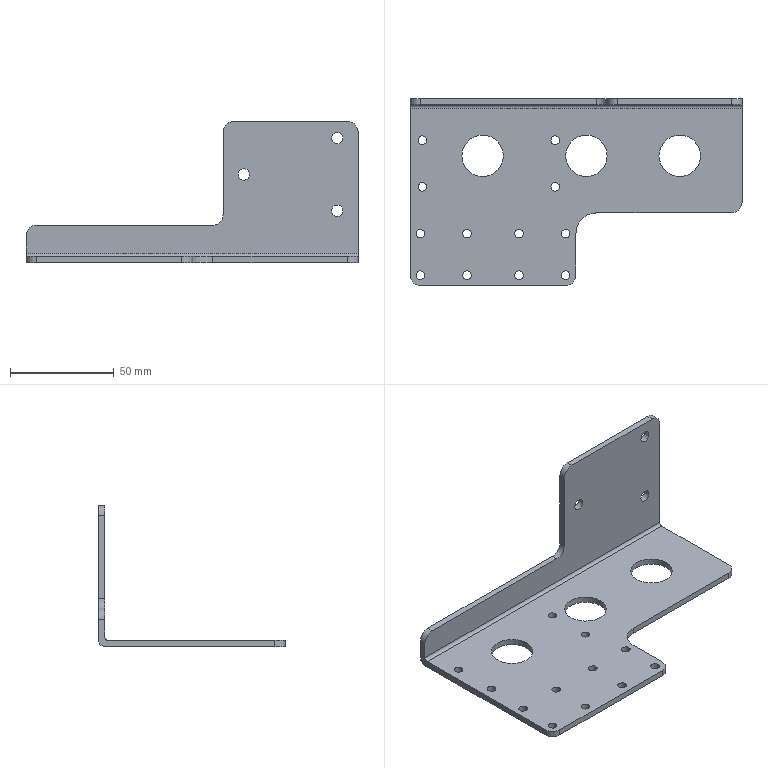Part | NX | 1 solid | 40 faces | box 160 x 90 x 68 mm | volume 47962 mm3 | cylinder 28 | plane 12 | commonest cylinder face diameters 4.2 x12 10 x7 20 x4 5.5 x3 3 x1 6 x1
STEP:
#1=CARTESIAN_POINT('',(-29.6,-57.5,1.5));
#2=VERTEX_POINT('',#1);
#3=CARTESIAN_POINT('',(-27.5,-57.5,1.5));
#4=DIRECTION('',(0.,0.,-1.));
#5=DIRECTION('',(-1.,0.,0.));
#6=AXIS2_PLACEMENT_3D('',#3,#4,#5);
#7=CIRCLE('',#6,2.1);
#8=EDGE_CURVE('',#2,#2,#7,.T.);
#9=ORIENTED_EDGE('',*,*,#8,.T.);
#10=EDGE_LOOP('',(#9));
#11=FACE_BOUND('',#10,.T.);
#12=CARTESIAN_POINT('',(-54.6,-57.5,1.5));
#13=VERTEX_POINT('',#12);
#14=CARTESIAN_POINT('',(-52.5,-57.5,1.5));
#15=DIRECTION('',(0.,0.,-1.));
#16=DIRECTION('',(-1.,0.,0.));
#17=AXIS2_PLACEMENT_3D('',#14,#15,#16);
#18=CIRCLE('',#17,2.1);
#19=EDGE_CURVE('',#13,#13,#18,.T.);
#20=ORIENTED_EDGE('',*,*,#19,.T.);
#21=EDGE_LOOP('',(#20));
#22=FACE_BOUND('',#21,.T.);
#23=CARTESIAN_POINT('',(-77.1,-57.5,1.5));
#24=VERTEX_POINT('',#23);
#25=CARTESIAN_POINT('',(-75.,-57.5,1.5));
#26=DIRECTION('',(0.,0.,-1.));
#27=DIRECTION('',(-1.,0.,0.));
#28=AXIS2_PLACEMENT_3D('',#25,#26,#27);
#29=CIRCLE('',#28,2.1);
#30=EDGE_CURVE('',#24,#24,#29,.T.);
#31=ORIENTED_EDGE('',*,*,#30,.T.);
#32=EDGE_LOOP('',(#31));
#33=FACE_BOUND('',#32,.T.);
#34=CARTESIAN_POINT('',(-7.1,-57.5,1.5));
#35=VERTEX_POINT('',#34);
#36=CARTESIAN_POINT('',(-5.,-57.5,1.5));
#37=DIRECTION('',(0.,0.,-1.));
#38=DIRECTION('',(-1.,0.,0.));
#39=AXIS2_PLACEMENT_3D('',#36,#37,#38);
#40=CIRCLE('',#39,2.1);
#41=EDGE_CURVE('',#35,#35,#40,.T.);
#42=ORIENTED_EDGE('',*,*,#41,.T.);
#43=EDGE_LOOP('',(#42));
#44=FACE_BOUND('',#43,.T.);
#45=CARTESIAN_POINT('',(-7.1,-37.5,1.5));
#46=VERTEX_POINT('',#45);
#47=CARTESIAN_POINT('',(-5.,-37.5,1.5));
#48=DIRECTION('',(0.,0.,-1.));
#49=DIRECTION('',(-1.,0.,0.));
#50=AXIS2_PLACEMENT_3D('',#47,#48,#49);
#51=CIRCLE('',#50,2.1);
#52=EDGE_CURVE('',#46,#46,#51,.T.);
#53=ORIENTED_EDGE('',*,*,#52,.T.);
#54=EDGE_LOOP('',(#53));
#55=FACE_BOUND('',#54,.T.);
#56=CARTESIAN_POINT('',(-29.6,-37.5,1.5));
#57=VERTEX_POINT('',#56);
#58=CARTESIAN_POINT('',(-27.5,-37.5,1.5));
#59=DIRECTION('',(0.,0.,-1.));
#60=DIRECTION('',(-1.,0.,0.));
#61=AXIS2_PLACEMENT_3D('',#58,#59,#60);
#62=CIRCLE('',#61,2.1);
#63=EDGE_CURVE('',#57,#57,#62,.T.);
#64=ORIENTED_EDGE('',*,*,#63,.T.);
#65=EDGE_LOOP('',(#64));
#66=FACE_BOUND('',#65,.T.);
#67=CARTESIAN_POINT('',(-54.6,-37.5,1.5));
#68=VERTEX_POINT('',#67);
#69=CARTESIAN_POINT('',(-52.5,-37.5,1.5));
#70=DIRECTION('',(0.,0.,-1.));
#71=DIRECTION('',(-1.,0.,0.));
#72=AXIS2_PLACEMENT_3D('',#69,#70,#71);
#73=CIRCLE('',#72,2.1);
#74=EDGE_CURVE('',#68,#68,#73,.T.);
#75=ORIENTED_EDGE('',*,*,#74,.T.);
#76=EDGE_LOOP('',(#75));
#77=FACE_BOUND('',#76,.T.);
#78=CARTESIAN_POINT('',(-77.1,-37.5,1.5));
#79=VERTEX_POINT('',#78);
#80=CARTESIAN_POINT('',(-75.,-37.5,1.5));
#81=DIRECTION('',(0.,0.,-1.));
#82=DIRECTION('',(-1.,0.,0.));
#83=AXIS2_PLACEMENT_3D('',#80,#81,#82);
#84=CIRCLE('',#83,2.1);
#85=EDGE_CURVE('',#79,#79,#84,.T.);
#86=ORIENTED_EDGE('',*,*,#85,.T.);
#87=EDGE_LOOP('',(#86));
#88=FACE_BOUND('',#87,.T.);
#89=CARTESIAN_POINT('',(-5.,0.,1.5));
#90=VERTEX_POINT('',#89);
#91=CARTESIAN_POINT('',(5.,0.,1.5));
#92=DIRECTION('',(0.,0.,-1.));
#93=DIRECTION('',(-1.,0.,0.));
#94=AXIS2_PLACEMENT_3D('',#91,#92,#93);
#95=CIRCLE('',#94,10.);
#96=EDGE_CURVE('',#90,#90,#95,.T.);
#97=ORIENTED_EDGE('',*,*,#96,.T.);
#98=EDGE_LOOP('',(#97));
#99=FACE_BOUND('',#98,.T.);
#100=CARTESIAN_POINT('',(-55.,0.,1.5));
#101=VERTEX_POINT('',#100);
#102=CARTESIAN_POINT('',(-45.,0.,1.5));
#103=DIRECTION('',(0.,0.,-1.));
#104=DIRECTION('',(-1.,0.,0.));
#105=AXIS2_PLACEMENT_3D('',#102,#103,#104);
#106=CIRCLE('',#105,10.);
#107=EDGE_CURVE('',#101,#101,#106,.T.);
#108=ORIENTED_EDGE('',*,*,#107,.T.);
#109=EDGE_LOOP('',(#108));
#110=FACE_BOUND('',#109,.T.);
#111=CARTESIAN_POINT('',(40.,0.,1.5));
#112=VERTEX_POINT('',#111);
#113=CARTESIAN_POINT('',(50.,0.,1.5));
#114=DIRECTION('',(0.,0.,-1.));
#115=DIRECTION('',(-1.,0.,0.));
#116=AXIS2_PLACEMENT_3D('',#113,#114,#115);
#117=CIRCLE('',#116,10.);
#118=EDGE_CURVE('',#112,#112,#117,.T.);
#119=ORIENTED_EDGE('',*,*,#118,.T.);
#120=EDGE_LOOP('',(#119));
#121=FACE_BOUND('',#120,.T.);
#122=CARTESIAN_POINT('',(-12.1,-15.,1.5));
#123=VERTEX_POINT('',#122);
#124=CARTESIAN_POINT('',(-10.,-15.,1.5));
#125=DIRECTION('',(0.,0.,-1.));
#126=DIRECTION('',(-1.,0.,0.));
#127=AXIS2_PLACEMENT_3D('',#124,#125,#126);
#128=CIRCLE('',#127,2.1);
#129=EDGE_CURVE('',#123,#123,#128,.T.);
#130=ORIENTED_EDGE('',*,*,#129,.T.);
#131=EDGE_LOOP('',(#130));
#132=FACE_BOUND('',#131,.T.);
#133=CARTESIAN_POINT('',(-76.1,-15.,1.5));
#134=VERTEX_POINT('',#133);
#135=CARTESIAN_POINT('',(-74.,-15.,1.5));
#136=DIRECTION('',(0.,0.,-1.));
#137=DIRECTION('',(-1.,0.,0.));
#138=AXIS2_PLACEMENT_3D('',#135,#136,#137);
#139=CIRCLE('',#138,2.1);
#140=EDGE_CURVE('',#134,#134,#139,.T.);
#141=ORIENTED_EDGE('',*,*,#140,.T.);
#142=EDGE_LOOP('',(#141));
#143=FACE_BOUND('',#142,.T.);
#144=CARTESIAN_POINT('',(-12.1,7.5,1.5));
#145=VERTEX_POINT('',#144);
#146=CARTESIAN_POINT('',(-10.,7.5,1.5));
#147=DIRECTION('',(0.,0.,-1.));
#148=DIRECTION('',(-1.,0.,0.));
#149=AXIS2_PLACEMENT_3D('',#146,#147,#148);
#150=CIRCLE('',#149,2.1);
#151=EDGE_CURVE('',#145,#145,#150,.T.);
#152=ORIENTED_EDGE('',*,*,#151,.T.);
#153=EDGE_LOOP('',(#152));
#154=FACE_BOUND('',#153,.T.);
#155=CARTESIAN_POINT('',(-76.1,7.5,1.5));
#156=VERTEX_POINT('',#155);
#157=CARTESIAN_POINT('',(-74.,7.5,1.5));
#158=DIRECTION('',(0.,0.,-1.));
#159=DIRECTION('',(-1.,0.,0.));
#160=AXIS2_PLACEMENT_3D('',#157,#158,#159);
#161=CIRCLE('',#160,2.1);
#162=EDGE_CURVE('',#156,#156,#161,.T.);
#163=ORIENTED_EDGE('',*,*,#162,.T.);
#164=EDGE_LOOP('',(#163));
#165=FACE_BOUND('',#164,.T.);
#166=CARTESIAN_POINT('',(80.,-22.5,1.5));
#167=VERTEX_POINT('',#166);
#168=CARTESIAN_POINT('',(80.,23.,1.5));
#169=VERTEX_POINT('',#168);
#170=CARTESIAN_POINT('',(80.,27.5,1.5));
#171=DIRECTION('',(0.,1.,0.));
#172=VECTOR('',#171,1000.);
#173=LINE('',#170,#172);
#174=EDGE_CURVE('',#167,#169,#173,.T.);
#175=ORIENTED_EDGE('',*,*,#174,.T.);
#176=CARTESIAN_POINT('',(-80.,23.,1.5));
#177=VERTEX_POINT('',#176);
#178=CARTESIAN_POINT('',(-80.,23.,1.5));
#179=DIRECTION('',(1.,0.,0.));
#180=VECTOR('',#179,1000.);
#181=LINE('',#178,#180);
#182=EDGE_CURVE('',#169,#177,#181,.F.);
#183=ORIENTED_EDGE('',*,*,#182,.T.);
#184=CARTESIAN_POINT('',(-80.,-57.5,1.5));
#185=VERTEX_POINT('',#184);
#186=CARTESIAN_POINT('',(-80.,27.5,1.5));
#187=DIRECTION('',(0.,-1.,0.));
#188=VECTOR('',#187,1000.);
#189=LINE('',#186,#188);
#190=EDGE_CURVE('',#177,#185,#189,.T.);
#191=ORIENTED_EDGE('',*,*,#190,.T.);
#192=CARTESIAN_POINT('',(-75.,-62.5,1.5));
#193=VERTEX_POINT('',#192);
#194=CARTESIAN_POINT('',(-75.,-57.5,1.5));
#195=DIRECTION('',(0.,0.,-1.));
#196=DIRECTION('',(-1.,0.,0.));
#197=AXIS2_PLACEMENT_3D('',#194,#195,#196);
#198=CIRCLE('',#197,5.);
#199=EDGE_CURVE('',#185,#193,#198,.F.);
#200=ORIENTED_EDGE('',*,*,#199,.T.);
#201=CARTESIAN_POINT('',(-5.,-62.5,1.5));
#202=VERTEX_POINT('',#201);
#203=CARTESIAN_POINT('',(-80.,-62.5,1.5));
#204=DIRECTION('',(1.,0.,0.));
#205=VECTOR('',#204,1000.);
#206=LINE('',#203,#205);
#207=EDGE_CURVE('',#193,#202,#206,.T.);
#208=ORIENTED_EDGE('',*,*,#207,.T.);
#209=CARTESIAN_POINT('',(0.,-57.5,1.5));
#210=VERTEX_POINT('',#209);
#211=CARTESIAN_POINT('',(-5.,-57.5,1.5));
#212=DIRECTION('',(0.,0.,-1.));
#213=DIRECTION('',(-1.,0.,0.));
#214=AXIS2_PLACEMENT_3D('',#211,#212,#213);
#215=CIRCLE('',#214,5.);
#216=EDGE_CURVE('',#202,#210,#215,.F.);
#217=ORIENTED_EDGE('',*,*,#216,.T.);
#218=CARTESIAN_POINT('',(0.,-37.5,1.5));
#219=VERTEX_POINT('',#218);
#220=CARTESIAN_POINT('',(0.,-27.5,1.5));
#221=DIRECTION('',(0.,1.,0.));
#222=VECTOR('',#221,1000.);
#223=LINE('',#220,#222);
#224=EDGE_CURVE('',#210,#219,#223,.T.);
#225=ORIENTED_EDGE('',*,*,#224,.T.);
#226=CARTESIAN_POINT('',(10.,-27.5,1.5));
#227=VERTEX_POINT('',#226);
#228=CARTESIAN_POINT('',(10.,-37.5,1.5));
#229=DIRECTION('',(0.,0.,-1.));
#230=DIRECTION('',(-1.,0.,0.));
#231=AXIS2_PLACEMENT_3D('',#228,#229,#230);
#232=CIRCLE('',#231,10.);
#233=EDGE_CURVE('',#219,#227,#232,.T.);
#234=ORIENTED_EDGE('',*,*,#233,.T.);
#235=CARTESIAN_POINT('',(75.,-27.5,1.5));
#236=VERTEX_POINT('',#235);
#237=CARTESIAN_POINT('',(80.,-27.5,1.5));
#238=DIRECTION('',(1.,0.,0.));
#239=VECTOR('',#238,1000.);
#240=LINE('',#237,#239);
#241=EDGE_CURVE('',#227,#236,#240,.T.);
#242=ORIENTED_EDGE('',*,*,#241,.T.);
#243=CARTESIAN_POINT('',(75.,-22.5,1.5));
#244=DIRECTION('',(0.,0.,-1.));
#245=DIRECTION('',(-1.,0.,0.));
#246=AXIS2_PLACEMENT_3D('',#243,#244,#245);
#247=CIRCLE('',#246,5.);
#248=EDGE_CURVE('',#236,#167,#247,.F.);
#249=ORIENTED_EDGE('',*,*,#248,.T.);
#250=EDGE_LOOP('',(#175,#183,#191,#200,#208,#217,#225,#234,#242,#249));
#251=FACE_BOUND('',#250,.T.);
#252=CARTESIAN_POINT('',(0.,0.,1.5));
#253=DIRECTION('',(0.,0.,-1.));
#254=DIRECTION('',(-1.,0.,0.));
#255=AXIS2_PLACEMENT_3D('',#252,#253,#254);
#256=PLANE('',#255);
#257=ADVANCED_FACE('',(#11,#22,#33,#44,#55,#66,#77,#88,#99,#110,#121,#132,#143,#154,#165,#251),#256,.F.);
#258=CARTESIAN_POINT('',(15.,27.5,61.5));
#259=VERTEX_POINT('',#258);
#260=CARTESIAN_POINT('',(15.,27.5,21.5));
#261=VERTEX_POINT('',#260);
#262=CARTESIAN_POINT('',(15.,27.5,66.5));
#263=DIRECTION('',(0.,0.,-1.));
#264=VECTOR('',#263,1000.);
#265=LINE('',#262,#264);
#266=EDGE_CURVE('',#259,#261,#265,.T.);
#267=ORIENTED_EDGE('',*,*,#266,.T.);
#268=CARTESIAN_POINT('',(15.,24.5,21.5));
#269=VERTEX_POINT('',#268);
#270=CARTESIAN_POINT('',(15.,24.5,21.5));
#271=DIRECTION('',(0.,1.,0.));
#272=VECTOR('',#271,1000.);
#273=LINE('',#270,#272);
#274=EDGE_CURVE('',#261,#269,#273,.F.);
#275=ORIENTED_EDGE('',*,*,#274,.T.);
#276=CARTESIAN_POINT('',(15.,24.5,61.5));
#277=VERTEX_POINT('',#276);
#278=CARTESIAN_POINT('',(15.,24.5,66.5));
#279=DIRECTION('',(0.,0.,-1.));
#280=VECTOR('',#279,1000.);
#281=LINE('',#278,#280);
#282=EDGE_CURVE('',#277,#269,#281,.T.);
#283=ORIENTED_EDGE('',*,*,#282,.F.);
#284=CARTESIAN_POINT('',(15.,27.5,61.5));
#285=DIRECTION('',(0.,-1.,0.));
#286=VECTOR('',#285,1000.);
#287=LINE('',#284,#286);
#288=EDGE_CURVE('',#277,#259,#287,.F.);
#289=ORIENTED_EDGE('',*,*,#288,.T.);
#290=EDGE_LOOP('',(#267,#275,#283,#289));
#291=FACE_BOUND('',#290,.T.);
#292=CARTESIAN_POINT('',(15.,27.5,66.5));
#293=DIRECTION('',(1.,0.,0.));
#294=DIRECTION('',(0.,1.,0.));
#295=AXIS2_PLACEMENT_3D('',#292,#293,#294);
#296=PLANE('',#295);
#297=ADVANCED_FACE('',(#291),#296,.F.);
#298=CARTESIAN_POINT('',(-80.,27.5,11.5));
#299=VERTEX_POINT('',#298);
#300=CARTESIAN_POINT('',(-80.,27.5,1.5));
#301=VERTEX_POINT('',#300);
#302=CARTESIAN_POINT('',(-80.,27.5,1.5));
#303=DIRECTION('',(0.,0.,-1.));
#304=VECTOR('',#303,1000.);
#305=LINE('',#302,#304);
#306=EDGE_CURVE('',#299,#301,#305,.T.);
#307=ORIENTED_EDGE('',*,*,#306,.T.);
#308=CARTESIAN_POINT('',(-80.,24.5,-1.5));
#309=VERTEX_POINT('',#308);
#310=CARTESIAN_POINT('',(-80.,24.5,1.5));
#311=DIRECTION('',(1.,0.,0.));
#312=DIRECTION('',(0.,0.,-1.));
#313=AXIS2_PLACEMENT_3D('',#310,#311,#312);
#314=CIRCLE('',#313,3.);
#315=EDGE_CURVE('',#301,#309,#314,.F.);
#316=ORIENTED_EDGE('',*,*,#315,.T.);
#317=CARTESIAN_POINT('',(-80.,-57.5,-1.5));
#318=VERTEX_POINT('',#317);
#319=CARTESIAN_POINT('',(-80.,27.5,-1.5));
#320=DIRECTION('',(0.,-1.,0.));
#321=VECTOR('',#320,1000.);
#322=LINE('',#319,#321);
#323=EDGE_CURVE('',#309,#318,#322,.T.);
#324=ORIENTED_EDGE('',*,*,#323,.T.);
#325=CARTESIAN_POINT('',(-80.,-57.5,1.5));
#326=DIRECTION('',(0.,0.,-1.));
#327=VECTOR('',#326,1000.);
#328=LINE('',#325,#327);
#329=EDGE_CURVE('',#318,#185,#328,.F.);
#330=ORIENTED_EDGE('',*,*,#329,.T.);
#331=ORIENTED_EDGE('',*,*,#190,.F.);
#332=CARTESIAN_POINT('',(-80.,24.5,3.));
#333=VERTEX_POINT('',#332);
#334=CARTESIAN_POINT('',(-80.,23.,3.));
#335=DIRECTION('',(1.,0.,0.));
#336=DIRECTION('',(0.,0.,-1.));
#337=AXIS2_PLACEMENT_3D('',#334,#335,#336);
#338=CIRCLE('',#337,1.5);
#339=EDGE_CURVE('',#177,#333,#338,.T.);
#340=ORIENTED_EDGE('',*,*,#339,.T.);
#341=CARTESIAN_POINT('',(-80.,24.5,11.5));
#342=VERTEX_POINT('',#341);
#343=CARTESIAN_POINT('',(-80.,24.5,1.5));
#344=DIRECTION('',(0.,0.,-1.));
#345=VECTOR('',#344,1000.);
#346=LINE('',#343,#345);
#347=EDGE_CURVE('',#342,#333,#346,.T.);
#348=ORIENTED_EDGE('',*,*,#347,.F.);
#349=CARTESIAN_POINT('',(-80.,27.5,11.5));
#350=DIRECTION('',(0.,-1.,0.));
#351=VECTOR('',#350,1000.);
#352=LINE('',#349,#351);
#353=EDGE_CURVE('',#342,#299,#352,.F.);
#354=ORIENTED_EDGE('',*,*,#353,.T.);
#355=EDGE_LOOP('',(#307,#316,#324,#330,#331,#340,#348,#354));
#356=FACE_BOUND('',#355,.T.);
#357=CARTESIAN_POINT('',(-80.,27.5,1.5));
#358=DIRECTION('',(1.,0.,0.));
#359=DIRECTION('',(0.,0.,-1.));
#360=AXIS2_PLACEMENT_3D('',#357,#358,#359);
#361=PLANE('',#360);
#362=ADVANCED_FACE('',(#356),#361,.F.);
#363=CARTESIAN_POINT('',(10.,-27.5,-1.5));
#364=VERTEX_POINT('',#363);
#365=CARTESIAN_POINT('',(75.,-27.5,-1.5));
#366=VERTEX_POINT('',#365);
#367=CARTESIAN_POINT('',(80.,-27.5,-1.5));
#368=DIRECTION('',(1.,0.,0.));
#369=VECTOR('',#368,1000.);
#370=LINE('',#367,#369);
#371=EDGE_CURVE('',#364,#366,#370,.T.);
#372=ORIENTED_EDGE('',*,*,#371,.T.);
#373=CARTESIAN_POINT('',(75.,-27.5,1.5));
#374=DIRECTION('',(0.,0.,-1.));
#375=VECTOR('',#374,1000.);
#376=LINE('',#373,#375);
#377=EDGE_CURVE('',#366,#236,#376,.F.);
#378=ORIENTED_EDGE('',*,*,#377,.T.);
#379=ORIENTED_EDGE('',*,*,#241,.F.);
#380=CARTESIAN_POINT('',(10.,-27.5,1.5));
#381=DIRECTION('',(0.,0.,-1.));
#382=VECTOR('',#381,1000.);
#383=LINE('',#380,#382);
#384=EDGE_CURVE('',#227,#364,#383,.T.);
#385=ORIENTED_EDGE('',*,*,#384,.T.);
#386=EDGE_LOOP('',(#372,#378,#379,#385));
#387=FACE_BOUND('',#386,.T.);
#388=CARTESIAN_POINT('',(80.,-27.5,1.5));
#389=DIRECTION('',(0.,1.,0.));
#390=DIRECTION('',(-1.,0.,0.));
#391=AXIS2_PLACEMENT_3D('',#388,#389,#390);
#392=PLANE('',#391);
#393=ADVANCED_FACE('',(#387),#392,.F.);
#394=CARTESIAN_POINT('',(80.,-22.5,-1.5));
#395=VERTEX_POINT('',#394);
#396=CARTESIAN_POINT('',(80.,24.5,-1.5));
#397=VERTEX_POINT('',#396);
#398=CARTESIAN_POINT('',(80.,27.5,-1.5));
#399=DIRECTION('',(0.,1.,0.));
#400=VECTOR('',#399,1000.);
#401=LINE('',#398,#400);
#402=EDGE_CURVE('',#395,#397,#401,.T.);
#403=ORIENTED_EDGE('',*,*,#402,.T.);
#404=CARTESIAN_POINT('',(80.,27.5,1.5));
#405=VERTEX_POINT('',#404);
#406=CARTESIAN_POINT('',(80.,24.5,1.5));
#407=DIRECTION('',(-1.,0.,0.));
#408=DIRECTION('',(0.,-1.,0.));
#409=AXIS2_PLACEMENT_3D('',#406,#407,#408);
#410=CIRCLE('',#409,3.);
#411=EDGE_CURVE('',#397,#405,#410,.F.);
#412=ORIENTED_EDGE('',*,*,#411,.T.);
#413=CARTESIAN_POINT('',(80.,27.5,61.5));
#414=VERTEX_POINT('',#413);
#415=CARTESIAN_POINT('',(80.,27.5,1.5));
#416=DIRECTION('',(0.,0.,-1.));
#417=VECTOR('',#416,1000.);
#418=LINE('',#415,#417);
#419=EDGE_CURVE('',#414,#405,#418,.T.);
#420=ORIENTED_EDGE('',*,*,#419,.F.);
#421=CARTESIAN_POINT('',(80.,24.5,61.5));
#422=VERTEX_POINT('',#421);
#423=CARTESIAN_POINT('',(80.,27.5,61.5));
#424=DIRECTION('',(0.,1.,0.));
#425=VECTOR('',#424,1000.);
#426=LINE('',#423,#425);
#427=EDGE_CURVE('',#414,#422,#426,.F.);
#428=ORIENTED_EDGE('',*,*,#427,.T.);
#429=CARTESIAN_POINT('',(80.,24.5,3.));
#430=VERTEX_POINT('',#429);
#431=CARTESIAN_POINT('',(80.,24.5,66.5));
#432=DIRECTION('',(0.,0.,-1.));
#433=VECTOR('',#432,1000.);
#434=LINE('',#431,#433);
#435=EDGE_CURVE('',#422,#430,#434,.T.);
#436=ORIENTED_EDGE('',*,*,#435,.T.);
#437=CARTESIAN_POINT('',(80.,23.,3.));
#438=DIRECTION('',(-1.,0.,0.));
#439=DIRECTION('',(0.,-1.,0.));
#440=AXIS2_PLACEMENT_3D('',#437,#438,#439);
#441=CIRCLE('',#440,1.5);
#442=EDGE_CURVE('',#430,#169,#441,.T.);
#443=ORIENTED_EDGE('',*,*,#442,.T.);
#444=ORIENTED_EDGE('',*,*,#174,.F.);
#445=CARTESIAN_POINT('',(80.,-22.5,1.5));
#446=DIRECTION('',(0.,0.,-1.));
#447=VECTOR('',#446,1000.);
#448=LINE('',#445,#447);
#449=EDGE_CURVE('',#167,#395,#448,.T.);
#450=ORIENTED_EDGE('',*,*,#449,.T.);
#451=EDGE_LOOP('',(#403,#412,#420,#428,#436,#443,#444,#450));
#452=FACE_BOUND('',#451,.T.);
#453=CARTESIAN_POINT('',(80.,27.5,1.5));
#454=DIRECTION('',(-1.,0.,0.));
#455=DIRECTION('',(0.,-1.,0.));
#456=AXIS2_PLACEMENT_3D('',#453,#454,#455);
#457=PLANE('',#456);
#458=ADVANCED_FACE('',(#452),#457,.F.);
#459=CARTESIAN_POINT('',(27.75,27.5,41.));
#460=VERTEX_POINT('',#459);
#461=CARTESIAN_POINT('',(25.,27.5,41.));
#462=DIRECTION('',(0.,-1.,0.));
#463=DIRECTION('',(1.,0.,0.));
#464=AXIS2_PLACEMENT_3D('',#461,#462,#463);
#465=CIRCLE('',#464,2.75);
#466=EDGE_CURVE('',#460,#460,#465,.T.);
#467=ORIENTED_EDGE('',*,*,#466,.T.);
#468=EDGE_LOOP('',(#467));
#469=FACE_BOUND('',#468,.T.);
#470=CARTESIAN_POINT('',(72.75,27.5,23.5));
#471=VERTEX_POINT('',#470);
#472=CARTESIAN_POINT('',(70.,27.5,23.5));
#473=DIRECTION('',(0.,-1.,0.));
#474=DIRECTION('',(1.,0.,0.));
#475=AXIS2_PLACEMENT_3D('',#472,#473,#474);
#476=CIRCLE('',#475,2.75);
#477=EDGE_CURVE('',#471,#471,#476,.T.);
#478=ORIENTED_EDGE('',*,*,#477,.T.);
#479=EDGE_LOOP('',(#478));
#480=FACE_BOUND('',#479,.T.);
#481=CARTESIAN_POINT('',(72.75,27.5,58.5));
#482=VERTEX_POINT('',#481);
#483=CARTESIAN_POINT('',(70.,27.5,58.5));
#484=DIRECTION('',(0.,-1.,0.));
#485=DIRECTION('',(1.,0.,0.));
#486=AXIS2_PLACEMENT_3D('',#483,#484,#485);
#487=CIRCLE('',#486,2.75);
#488=EDGE_CURVE('',#482,#482,#487,.T.);
#489=ORIENTED_EDGE('',*,*,#488,.T.);
#490=EDGE_LOOP('',(#489));
#491=FACE_BOUND('',#490,.T.);
#492=ORIENTED_EDGE('',*,*,#419,.T.);
#493=CARTESIAN_POINT('',(-80.,27.5,1.5));
#494=DIRECTION('',(-1.,0.,0.));
#495=VECTOR('',#494,1000.);
#496=LINE('',#493,#495);
#497=EDGE_CURVE('',#405,#301,#496,.T.);
#498=ORIENTED_EDGE('',*,*,#497,.T.);
#499=ORIENTED_EDGE('',*,*,#306,.F.);
#500=CARTESIAN_POINT('',(-75.,27.5,16.5));
#501=VERTEX_POINT('',#500);
#502=CARTESIAN_POINT('',(-75.,27.5,11.5));
#503=DIRECTION('',(0.,-1.,0.));
#504=DIRECTION('',(1.,0.,0.));
#505=AXIS2_PLACEMENT_3D('',#502,#503,#504);
#506=CIRCLE('',#505,5.);
#507=EDGE_CURVE('',#299,#501,#506,.F.);
#508=ORIENTED_EDGE('',*,*,#507,.T.);
#509=CARTESIAN_POINT('',(10.,27.5,16.5));
#510=VERTEX_POINT('',#509);
#511=CARTESIAN_POINT('',(-95.297,27.5,16.5));
#512=DIRECTION('',(1.,0.,0.));
#513=VECTOR('',#512,1000.);
#514=LINE('',#511,#513);
#515=EDGE_CURVE('',#501,#510,#514,.T.);
#516=ORIENTED_EDGE('',*,*,#515,.T.);
#517=CARTESIAN_POINT('',(10.,27.5,21.5));
#518=DIRECTION('',(0.,-1.,0.));
#519=DIRECTION('',(1.,0.,0.));
#520=AXIS2_PLACEMENT_3D('',#517,#518,#519);
#521=CIRCLE('',#520,5.);
#522=EDGE_CURVE('',#510,#261,#521,.T.);
#523=ORIENTED_EDGE('',*,*,#522,.T.);
#524=ORIENTED_EDGE('',*,*,#266,.F.);
#525=CARTESIAN_POINT('',(20.,27.5,66.5));
#526=VERTEX_POINT('',#525);
#527=CARTESIAN_POINT('',(20.,27.5,61.5));
#528=DIRECTION('',(0.,-1.,0.));
#529=DIRECTION('',(1.,0.,0.));
#530=AXIS2_PLACEMENT_3D('',#527,#528,#529);
#531=CIRCLE('',#530,5.);
#532=EDGE_CURVE('',#259,#526,#531,.F.);
#533=ORIENTED_EDGE('',*,*,#532,.T.);
#534=CARTESIAN_POINT('',(75.,27.5,66.5));
#535=VERTEX_POINT('',#534);
#536=CARTESIAN_POINT('',(80.,27.5,66.5));
#537=DIRECTION('',(-1.,0.,0.));
#538=VECTOR('',#537,1000.);
#539=LINE('',#536,#538);
#540=EDGE_CURVE('',#535,#526,#539,.T.);
#541=ORIENTED_EDGE('',*,*,#540,.F.);
#542=CARTESIAN_POINT('',(75.,27.5,61.5));
#543=DIRECTION('',(0.,-1.,0.));
#544=DIRECTION('',(1.,0.,0.));
#545=AXIS2_PLACEMENT_3D('',#542,#543,#544);
#546=CIRCLE('',#545,5.);
#547=EDGE_CURVE('',#535,#414,#546,.F.);
#548=ORIENTED_EDGE('',*,*,#547,.T.);
#549=EDGE_LOOP('',(#492,#498,#499,#508,#516,#523,#524,#533,#541,#548));
#550=FACE_BOUND('',#549,.T.);
#551=CARTESIAN_POINT('',(80.,27.5,1.5));
#552=DIRECTION('',(0.,-1.,0.));
#553=DIRECTION('',(1.,0.,0.));
#554=AXIS2_PLACEMENT_3D('',#551,#552,#553);
#555=PLANE('',#554);
#556=ADVANCED_FACE('',(#469,#480,#491,#550),#555,.F.);
#557=CARTESIAN_POINT('',(-29.6,-57.5,-1.5));
#558=VERTEX_POINT('',#557);
#559=CARTESIAN_POINT('',(-27.5,-57.5,-1.5));
#560=DIRECTION('',(0.,0.,-1.));
#561=DIRECTION('',(-1.,0.,0.));
#562=AXIS2_PLACEMENT_3D('',#559,#560,#561);
#563=CIRCLE('',#562,2.1);
#564=EDGE_CURVE('',#558,#558,#563,.T.);
#565=ORIENTED_EDGE('',*,*,#564,.F.);
#566=EDGE_LOOP('',(#565));
#567=FACE_BOUND('',#566,.T.);
#568=CARTESIAN_POINT('',(-54.6,-57.5,-1.5));
#569=VERTEX_POINT('',#568);
#570=CARTESIAN_POINT('',(-52.5,-57.5,-1.5));
#571=DIRECTION('',(0.,0.,-1.));
#572=DIRECTION('',(-1.,0.,0.));
#573=AXIS2_PLACEMENT_3D('',#570,#571,#572);
#574=CIRCLE('',#573,2.1);
#575=EDGE_CURVE('',#569,#569,#574,.T.);
#576=ORIENTED_EDGE('',*,*,#575,.F.);
#577=EDGE_LOOP('',(#576));
#578=FACE_BOUND('',#577,.T.);
#579=CARTESIAN_POINT('',(-77.1,-57.5,-1.5));
#580=VERTEX_POINT('',#579);
#581=CARTESIAN_POINT('',(-75.,-57.5,-1.5));
#582=DIRECTION('',(0.,0.,-1.));
#583=DIRECTION('',(-1.,0.,0.));
#584=AXIS2_PLACEMENT_3D('',#581,#582,#583);
#585=CIRCLE('',#584,2.1);
#586=EDGE_CURVE('',#580,#580,#585,.T.);
#587=ORIENTED_EDGE('',*,*,#586,.F.);
#588=EDGE_LOOP('',(#587));
#589=FACE_BOUND('',#588,.T.);
#590=CARTESIAN_POINT('',(-7.1,-57.5,-1.5));
#591=VERTEX_POINT('',#590);
#592=CARTESIAN_POINT('',(-5.,-57.5,-1.5));
#593=DIRECTION('',(0.,0.,-1.));
#594=DIRECTION('',(-1.,0.,0.));
#595=AXIS2_PLACEMENT_3D('',#592,#593,#594);
#596=CIRCLE('',#595,2.1);
#597=EDGE_CURVE('',#591,#591,#596,.T.);
#598=ORIENTED_EDGE('',*,*,#597,.F.);
#599=EDGE_LOOP('',(#598));
#600=FACE_BOUND('',#599,.T.);
#601=CARTESIAN_POINT('',(-7.1,-37.5,-1.5));
#602=VERTEX_POINT('',#601);
#603=CARTESIAN_POINT('',(-5.,-37.5,-1.5));
#604=DIRECTION('',(0.,0.,-1.));
#605=DIRECTION('',(-1.,0.,0.));
#606=AXIS2_PLACEMENT_3D('',#603,#604,#605);
#607=CIRCLE('',#606,2.1);
#608=EDGE_CURVE('',#602,#602,#607,.T.);
#609=ORIENTED_EDGE('',*,*,#608,.F.);
#610=EDGE_LOOP('',(#609));
#611=FACE_BOUND('',#610,.T.);
#612=CARTESIAN_POINT('',(-29.6,-37.5,-1.5));
#613=VERTEX_POINT('',#612);
#614=CARTESIAN_POINT('',(-27.5,-37.5,-1.5));
#615=DIRECTION('',(0.,0.,-1.));
#616=DIRECTION('',(-1.,0.,0.));
#617=AXIS2_PLACEMENT_3D('',#614,#615,#616);
#618=CIRCLE('',#617,2.1);
#619=EDGE_CURVE('',#613,#613,#618,.T.);
#620=ORIENTED_EDGE('',*,*,#619,.F.);
#621=EDGE_LOOP('',(#620));
#622=FACE_BOUND('',#621,.T.);
#623=CARTESIAN_POINT('',(-54.6,-37.5,-1.5));
#624=VERTEX_POINT('',#623);
#625=CARTESIAN_POINT('',(-52.5,-37.5,-1.5));
#626=DIRECTION('',(0.,0.,-1.));
#627=DIRECTION('',(-1.,0.,0.));
#628=AXIS2_PLACEMENT_3D('',#625,#626,#627);
#629=CIRCLE('',#628,2.1);
#630=EDGE_CURVE('',#624,#624,#629,.T.);
#631=ORIENTED_EDGE('',*,*,#630,.F.);
#632=EDGE_LOOP('',(#631));
#633=FACE_BOUND('',#632,.T.);
#634=CARTESIAN_POINT('',(-77.1,-37.5,-1.5));
#635=VERTEX_POINT('',#634);
#636=CARTESIAN_POINT('',(-75.,-37.5,-1.5));
#637=DIRECTION('',(0.,0.,-1.));
#638=DIRECTION('',(-1.,0.,0.));
#639=AXIS2_PLACEMENT_3D('',#636,#637,#638);
#640=CIRCLE('',#639,2.1);
#641=EDGE_CURVE('',#635,#635,#640,.T.);
#642=ORIENTED_EDGE('',*,*,#641,.F.);
#643=EDGE_LOOP('',(#642));
#644=FACE_BOUND('',#643,.T.);
#645=CARTESIAN_POINT('',(-5.,0.,-1.5));
#646=VERTEX_POINT('',#645);
#647=CARTESIAN_POINT('',(5.,0.,-1.5));
#648=DIRECTION('',(0.,0.,-1.));
#649=DIRECTION('',(-1.,0.,0.));
#650=AXIS2_PLACEMENT_3D('',#647,#648,#649);
#651=CIRCLE('',#650,10.);
#652=EDGE_CURVE('',#646,#646,#651,.T.);
#653=ORIENTED_EDGE('',*,*,#652,.F.);
#654=EDGE_LOOP('',(#653));
#655=FACE_BOUND('',#654,.T.);
#656=CARTESIAN_POINT('',(-55.,0.,-1.5));
#657=VERTEX_POINT('',#656);
#658=CARTESIAN_POINT('',(-45.,0.,-1.5));
#659=DIRECTION('',(0.,0.,-1.));
#660=DIRECTION('',(-1.,0.,0.));
#661=AXIS2_PLACEMENT_3D('',#658,#659,#660);
#662=CIRCLE('',#661,10.);
#663=EDGE_CURVE('',#657,#657,#662,.T.);
#664=ORIENTED_EDGE('',*,*,#663,.F.);
#665=EDGE_LOOP('',(#664));
#666=FACE_BOUND('',#665,.T.);
#667=CARTESIAN_POINT('',(40.,0.,-1.5));
#668=VERTEX_POINT('',#667);
#669=CARTESIAN_POINT('',(50.,0.,-1.5));
#670=DIRECTION('',(0.,0.,-1.));
#671=DIRECTION('',(-1.,0.,0.));
#672=AXIS2_PLACEMENT_3D('',#669,#670,#671);
#673=CIRCLE('',#672,10.);
#674=EDGE_CURVE('',#668,#668,#673,.T.);
#675=ORIENTED_EDGE('',*,*,#674,.F.);
#676=EDGE_LOOP('',(#675));
#677=FACE_BOUND('',#676,.T.);
#678=CARTESIAN_POINT('',(-12.1,-15.,-1.5));
#679=VERTEX_POINT('',#678);
#680=CARTESIAN_POINT('',(-10.,-15.,-1.5));
#681=DIRECTION('',(0.,0.,-1.));
#682=DIRECTION('',(-1.,0.,0.));
#683=AXIS2_PLACEMENT_3D('',#680,#681,#682);
#684=CIRCLE('',#683,2.1);
#685=EDGE_CURVE('',#679,#679,#684,.T.);
#686=ORIENTED_EDGE('',*,*,#685,.F.);
#687=EDGE_LOOP('',(#686));
#688=FACE_BOUND('',#687,.T.);
#689=CARTESIAN_POINT('',(-76.1,-15.,-1.5));
#690=VERTEX_POINT('',#689);
#691=CARTESIAN_POINT('',(-74.,-15.,-1.5));
#692=DIRECTION('',(0.,0.,-1.));
#693=DIRECTION('',(-1.,0.,0.));
#694=AXIS2_PLACEMENT_3D('',#691,#692,#693);
#695=CIRCLE('',#694,2.1);
#696=EDGE_CURVE('',#690,#690,#695,.T.);
#697=ORIENTED_EDGE('',*,*,#696,.F.);
#698=EDGE_LOOP('',(#697));
#699=FACE_BOUND('',#698,.T.);
#700=CARTESIAN_POINT('',(-12.1,7.5,-1.5));
#701=VERTEX_POINT('',#700);
#702=CARTESIAN_POINT('',(-10.,7.5,-1.5));
#703=DIRECTION('',(0.,0.,-1.));
#704=DIRECTION('',(-1.,0.,0.));
#705=AXIS2_PLACEMENT_3D('',#702,#703,#704);
#706=CIRCLE('',#705,2.1);
#707=EDGE_CURVE('',#701,#701,#706,.T.);
#708=ORIENTED_EDGE('',*,*,#707,.F.);
#709=EDGE_LOOP('',(#708));
#710=FACE_BOUND('',#709,.T.);
#711=CARTESIAN_POINT('',(-76.1,7.5,-1.5));
#712=VERTEX_POINT('',#711);
#713=CARTESIAN_POINT('',(-74.,7.5,-1.5));
#714=DIRECTION('',(0.,0.,-1.));
#715=DIRECTION('',(-1.,0.,0.));
#716=AXIS2_PLACEMENT_3D('',#713,#714,#715);
#717=CIRCLE('',#716,2.1);
#718=EDGE_CURVE('',#712,#712,#717,.T.);
#719=ORIENTED_EDGE('',*,*,#718,.F.);
#720=EDGE_LOOP('',(#719));
#721=FACE_BOUND('',#720,.T.);
#722=ORIENTED_EDGE('',*,*,#323,.F.);
#723=CARTESIAN_POINT('',(80.,24.5,-1.5));
#724=DIRECTION('',(-1.,0.,0.));
#725=VECTOR('',#724,1000.);
#726=LINE('',#723,#725);
#727=EDGE_CURVE('',#309,#397,#726,.F.);
#728=ORIENTED_EDGE('',*,*,#727,.T.);
#729=ORIENTED_EDGE('',*,*,#402,.F.);
#730=CARTESIAN_POINT('',(75.,-22.5,-1.5));
#731=DIRECTION('',(0.,0.,-1.));
#732=DIRECTION('',(-1.,0.,0.));
#733=AXIS2_PLACEMENT_3D('',#730,#731,#732);
#734=CIRCLE('',#733,5.);
#735=EDGE_CURVE('',#395,#366,#734,.T.);
#736=ORIENTED_EDGE('',*,*,#735,.T.);
#737=ORIENTED_EDGE('',*,*,#371,.F.);
#738=CARTESIAN_POINT('',(0.,-37.5,-1.5));
#739=VERTEX_POINT('',#738);
#740=CARTESIAN_POINT('',(10.,-37.5,-1.5));
#741=DIRECTION('',(0.,0.,-1.));
#742=DIRECTION('',(-1.,0.,0.));
#743=AXIS2_PLACEMENT_3D('',#740,#741,#742);
#744=CIRCLE('',#743,10.);
#745=EDGE_CURVE('',#364,#739,#744,.F.);
#746=ORIENTED_EDGE('',*,*,#745,.T.);
#747=CARTESIAN_POINT('',(0.,-57.5,-1.5));
#748=VERTEX_POINT('',#747);
#749=CARTESIAN_POINT('',(0.,-27.5,-1.5));
#750=DIRECTION('',(0.,-1.,0.));
#751=VECTOR('',#750,1000.);
#752=LINE('',#749,#751);
#753=EDGE_CURVE('',#739,#748,#752,.T.);
#754=ORIENTED_EDGE('',*,*,#753,.T.);
#755=CARTESIAN_POINT('',(-5.,-62.5,-1.5));
#756=VERTEX_POINT('',#755);
#757=CARTESIAN_POINT('',(-5.,-57.5,-1.5));
#758=DIRECTION('',(0.,0.,-1.));
#759=DIRECTION('',(-1.,0.,0.));
#760=AXIS2_PLACEMENT_3D('',#757,#758,#759);
#761=CIRCLE('',#760,5.);
#762=EDGE_CURVE('',#748,#756,#761,.T.);
#763=ORIENTED_EDGE('',*,*,#762,.T.);
#764=CARTESIAN_POINT('',(-75.,-62.5,-1.5));
#765=VERTEX_POINT('',#764);
#766=CARTESIAN_POINT('',(-80.,-62.5,-1.5));
#767=DIRECTION('',(-1.,0.,0.));
#768=VECTOR('',#767,1000.);
#769=LINE('',#766,#768);
#770=EDGE_CURVE('',#756,#765,#769,.T.);
#771=ORIENTED_EDGE('',*,*,#770,.T.);
#772=CARTESIAN_POINT('',(-75.,-57.5,-1.5));
#773=DIRECTION('',(0.,0.,-1.));
#774=DIRECTION('',(-1.,0.,0.));
#775=AXIS2_PLACEMENT_3D('',#772,#773,#774);
#776=CIRCLE('',#775,5.);
#777=EDGE_CURVE('',#765,#318,#776,.T.);
#778=ORIENTED_EDGE('',*,*,#777,.T.);
#779=EDGE_LOOP('',(#722,#728,#729,#736,#737,#746,#754,#763,#771,#778));
#780=FACE_BOUND('',#779,.T.);
#781=CARTESIAN_POINT('',(0.,0.,-1.5));
#782=DIRECTION('',(0.,0.,-1.));
#783=DIRECTION('',(-1.,0.,0.));
#784=AXIS2_PLACEMENT_3D('',#781,#782,#783);
#785=PLANE('',#784);
#786=ADVANCED_FACE('',(#567,#578,#589,#600,#611,#622,#633,#644,#655,#666,#677,#688,#699,#710,#721,#780),#785,.T.);
#787=ORIENTED_EDGE('',*,*,#718,.T.);
#788=EDGE_LOOP('',(#787));
#789=FACE_BOUND('',#788,.T.);
#790=ORIENTED_EDGE('',*,*,#162,.F.);
#791=EDGE_LOOP('',(#790));
#792=FACE_BOUND('',#791,.T.);
#793=CARTESIAN_POINT('',(-74.,7.5,-1.5));
#794=DIRECTION('',(0.,0.,-1.));
#795=DIRECTION('',(-1.,0.,0.));
#796=AXIS2_PLACEMENT_3D('',#793,#794,#795);
#797=CYLINDRICAL_SURFACE('',#796,2.1);
#798=ADVANCED_FACE('',(#789,#792),#797,.F.);
#799=ORIENTED_EDGE('',*,*,#707,.T.);
#800=EDGE_LOOP('',(#799));
#801=FACE_BOUND('',#800,.T.);
#802=ORIENTED_EDGE('',*,*,#151,.F.);
#803=EDGE_LOOP('',(#802));
#804=FACE_BOUND('',#803,.T.);
#805=CARTESIAN_POINT('',(-10.,7.5,-1.5));
#806=DIRECTION('',(0.,0.,-1.));
#807=DIRECTION('',(-1.,0.,0.));
#808=AXIS2_PLACEMENT_3D('',#805,#806,#807);
#809=CYLINDRICAL_SURFACE('',#808,2.1);
#810=ADVANCED_FACE('',(#801,#804),#809,.F.);
#811=ORIENTED_EDGE('',*,*,#696,.T.);
#812=EDGE_LOOP('',(#811));
#813=FACE_BOUND('',#812,.T.);
#814=ORIENTED_EDGE('',*,*,#140,.F.);
#815=EDGE_LOOP('',(#814));
#816=FACE_BOUND('',#815,.T.);
#817=CARTESIAN_POINT('',(-74.,-15.,-1.5));
#818=DIRECTION('',(0.,0.,-1.));
#819=DIRECTION('',(-1.,0.,0.));
#820=AXIS2_PLACEMENT_3D('',#817,#818,#819);
#821=CYLINDRICAL_SURFACE('',#820,2.1);
#822=ADVANCED_FACE('',(#813,#816),#821,.F.);
#823=ORIENTED_EDGE('',*,*,#685,.T.);
#824=EDGE_LOOP('',(#823));
#825=FACE_BOUND('',#824,.T.);
#826=ORIENTED_EDGE('',*,*,#129,.F.);
#827=EDGE_LOOP('',(#826));
#828=FACE_BOUND('',#827,.T.);
#829=CARTESIAN_POINT('',(-10.,-15.,-1.5));
#830=DIRECTION('',(0.,0.,-1.));
#831=DIRECTION('',(-1.,0.,0.));
#832=AXIS2_PLACEMENT_3D('',#829,#830,#831);
#833=CYLINDRICAL_SURFACE('',#832,2.1);
#834=ADVANCED_FACE('',(#825,#828),#833,.F.);
#835=ORIENTED_EDGE('',*,*,#118,.F.);
#836=EDGE_LOOP('',(#835));
#837=FACE_BOUND('',#836,.T.);
#838=ORIENTED_EDGE('',*,*,#674,.T.);
#839=EDGE_LOOP('',(#838));
#840=FACE_BOUND('',#839,.T.);
#841=CARTESIAN_POINT('',(50.,0.,1.5));
#842=DIRECTION('',(0.,0.,-1.));
#843=DIRECTION('',(-1.,0.,0.));
#844=AXIS2_PLACEMENT_3D('',#841,#842,#843);
#845=CYLINDRICAL_SURFACE('',#844,10.);
#846=ADVANCED_FACE('',(#837,#840),#845,.F.);
#847=ORIENTED_EDGE('',*,*,#107,.F.);
#848=EDGE_LOOP('',(#847));
#849=FACE_BOUND('',#848,.T.);
#850=ORIENTED_EDGE('',*,*,#663,.T.);
#851=EDGE_LOOP('',(#850));
#852=FACE_BOUND('',#851,.T.);
#853=CARTESIAN_POINT('',(-45.,0.,1.5));
#854=DIRECTION('',(0.,0.,-1.));
#855=DIRECTION('',(-1.,0.,0.));
#856=AXIS2_PLACEMENT_3D('',#853,#854,#855);
#857=CYLINDRICAL_SURFACE('',#856,10.);
#858=ADVANCED_FACE('',(#849,#852),#857,.F.);
#859=ORIENTED_EDGE('',*,*,#96,.F.);
#860=EDGE_LOOP('',(#859));
#861=FACE_BOUND('',#860,.T.);
#862=ORIENTED_EDGE('',*,*,#652,.T.);
#863=EDGE_LOOP('',(#862));
#864=FACE_BOUND('',#863,.T.);
#865=CARTESIAN_POINT('',(5.,0.,1.5));
#866=DIRECTION('',(0.,0.,-1.));
#867=DIRECTION('',(-1.,0.,0.));
#868=AXIS2_PLACEMENT_3D('',#865,#866,#867);
#869=CYLINDRICAL_SURFACE('',#868,10.);
#870=ADVANCED_FACE('',(#861,#864),#869,.F.);
#871=ORIENTED_EDGE('',*,*,#207,.F.);
#872=CARTESIAN_POINT('',(-75.,-62.5,-1.5));
#873=DIRECTION('',(0.,0.,-1.));
#874=VECTOR('',#873,1000.);
#875=LINE('',#872,#874);
#876=EDGE_CURVE('',#193,#765,#875,.T.);
#877=ORIENTED_EDGE('',*,*,#876,.T.);
#878=ORIENTED_EDGE('',*,*,#770,.F.);
#879=CARTESIAN_POINT('',(-5.,-62.5,88.821));
#880=DIRECTION('',(0.,0.,-1.));
#881=VECTOR('',#880,1000.);
#882=LINE('',#879,#881);
#883=EDGE_CURVE('',#756,#202,#882,.F.);
#884=ORIENTED_EDGE('',*,*,#883,.T.);
#885=EDGE_LOOP('',(#871,#877,#878,#884));
#886=FACE_BOUND('',#885,.T.);
#887=CARTESIAN_POINT('',(-80.,-62.5,88.821));
#888=DIRECTION('',(0.,-1.,0.));
#889=DIRECTION('',(1.,0.,0.));
#890=AXIS2_PLACEMENT_3D('',#887,#888,#889);
#891=PLANE('',#890);
#892=ADVANCED_FACE('',(#886),#891,.T.);
#893=ORIENTED_EDGE('',*,*,#224,.F.);
#894=CARTESIAN_POINT('',(0.,-57.5,88.821));
#895=DIRECTION('',(0.,0.,-1.));
#896=VECTOR('',#895,1000.);
#897=LINE('',#894,#896);
#898=EDGE_CURVE('',#210,#748,#897,.T.);
#899=ORIENTED_EDGE('',*,*,#898,.T.);
#900=ORIENTED_EDGE('',*,*,#753,.F.);
#901=CARTESIAN_POINT('',(0.,-37.5,88.821));
#902=DIRECTION('',(0.,0.,-1.));
#903=VECTOR('',#902,1000.);
#904=LINE('',#901,#903);
#905=EDGE_CURVE('',#739,#219,#904,.F.);
#906=ORIENTED_EDGE('',*,*,#905,.T.);
#907=EDGE_LOOP('',(#893,#899,#900,#906));
#908=FACE_BOUND('',#907,.T.);
#909=CARTESIAN_POINT('',(0.,-27.5,88.821));
#910=DIRECTION('',(1.,0.,0.));
#911=DIRECTION('',(0.,1.,0.));
#912=AXIS2_PLACEMENT_3D('',#909,#910,#911);
#913=PLANE('',#912);
#914=ADVANCED_FACE('',(#908),#913,.T.);
#915=ORIENTED_EDGE('',*,*,#233,.F.);
#916=ORIENTED_EDGE('',*,*,#905,.F.);
#917=ORIENTED_EDGE('',*,*,#745,.F.);
#918=ORIENTED_EDGE('',*,*,#384,.F.);
#919=EDGE_LOOP('',(#915,#916,#917,#918));
#920=FACE_BOUND('',#919,.T.);
#921=CARTESIAN_POINT('',(10.,-37.5,1.5));
#922=DIRECTION('',(0.,0.,-1.));
#923=DIRECTION('',(-1.,0.,0.));
#924=AXIS2_PLACEMENT_3D('',#921,#922,#923);
#925=CYLINDRICAL_SURFACE('',#924,10.);
#926=ADVANCED_FACE('',(#920),#925,.F.);
#927=ORIENTED_EDGE('',*,*,#641,.T.);
#928=EDGE_LOOP('',(#927));
#929=FACE_BOUND('',#928,.T.);
#930=ORIENTED_EDGE('',*,*,#85,.F.);
#931=EDGE_LOOP('',(#930));
#932=FACE_BOUND('',#931,.T.);
#933=CARTESIAN_POINT('',(-75.,-37.5,-1.5));
#934=DIRECTION('',(0.,0.,-1.));
#935=DIRECTION('',(-1.,0.,0.));
#936=AXIS2_PLACEMENT_3D('',#933,#934,#935);
#937=CYLINDRICAL_SURFACE('',#936,2.1);
#938=ADVANCED_FACE('',(#929,#932),#937,.F.);
#939=ORIENTED_EDGE('',*,*,#630,.T.);
#940=EDGE_LOOP('',(#939));
#941=FACE_BOUND('',#940,.T.);
#942=ORIENTED_EDGE('',*,*,#74,.F.);
#943=EDGE_LOOP('',(#942));
#944=FACE_BOUND('',#943,.T.);
#945=CARTESIAN_POINT('',(-52.5,-37.5,-1.5));
#946=DIRECTION('',(0.,0.,-1.));
#947=DIRECTION('',(-1.,0.,0.));
#948=AXIS2_PLACEMENT_3D('',#945,#946,#947);
#949=CYLINDRICAL_SURFACE('',#948,2.1);
#950=ADVANCED_FACE('',(#941,#944),#949,.F.);
#951=ORIENTED_EDGE('',*,*,#619,.T.);
#952=EDGE_LOOP('',(#951));
#953=FACE_BOUND('',#952,.T.);
#954=ORIENTED_EDGE('',*,*,#63,.F.);
#955=EDGE_LOOP('',(#954));
#956=FACE_BOUND('',#955,.T.);
#957=CARTESIAN_POINT('',(-27.5,-37.5,-1.5));
#958=DIRECTION('',(0.,0.,-1.));
#959=DIRECTION('',(-1.,0.,0.));
#960=AXIS2_PLACEMENT_3D('',#957,#958,#959);
#961=CYLINDRICAL_SURFACE('',#960,2.1);
#962=ADVANCED_FACE('',(#953,#956),#961,.F.);
#963=ORIENTED_EDGE('',*,*,#608,.T.);
#964=EDGE_LOOP('',(#963));
#965=FACE_BOUND('',#964,.T.);
#966=ORIENTED_EDGE('',*,*,#52,.F.);
#967=EDGE_LOOP('',(#966));
#968=FACE_BOUND('',#967,.T.);
#969=CARTESIAN_POINT('',(-5.,-37.5,-1.5));
#970=DIRECTION('',(0.,0.,-1.));
#971=DIRECTION('',(-1.,0.,0.));
#972=AXIS2_PLACEMENT_3D('',#969,#970,#971);
#973=CYLINDRICAL_SURFACE('',#972,2.1);
#974=ADVANCED_FACE('',(#965,#968),#973,.F.);
#975=ORIENTED_EDGE('',*,*,#597,.T.);
#976=EDGE_LOOP('',(#975));
#977=FACE_BOUND('',#976,.T.);
#978=ORIENTED_EDGE('',*,*,#41,.F.);
#979=EDGE_LOOP('',(#978));
#980=FACE_BOUND('',#979,.T.);
#981=CARTESIAN_POINT('',(-5.,-57.5,-1.5));
#982=DIRECTION('',(0.,0.,-1.));
#983=DIRECTION('',(-1.,0.,0.));
#984=AXIS2_PLACEMENT_3D('',#981,#982,#983);
#985=CYLINDRICAL_SURFACE('',#984,2.1);
#986=ADVANCED_FACE('',(#977,#980),#985,.F.);
#987=ORIENTED_EDGE('',*,*,#586,.T.);
#988=EDGE_LOOP('',(#987));
#989=FACE_BOUND('',#988,.T.);
#990=ORIENTED_EDGE('',*,*,#30,.F.);
#991=EDGE_LOOP('',(#990));
#992=FACE_BOUND('',#991,.T.);
#993=CARTESIAN_POINT('',(-75.,-57.5,-1.5));
#994=DIRECTION('',(0.,0.,-1.));
#995=DIRECTION('',(-1.,0.,0.));
#996=AXIS2_PLACEMENT_3D('',#993,#994,#995);
#997=CYLINDRICAL_SURFACE('',#996,2.1);
#998=ADVANCED_FACE('',(#989,#992),#997,.F.);
#999=ORIENTED_EDGE('',*,*,#575,.T.);
#1000=EDGE_LOOP('',(#999));
#1001=FACE_BOUND('',#1000,.T.);
#1002=ORIENTED_EDGE('',*,*,#19,.F.);
#1003=EDGE_LOOP('',(#1002));
#1004=FACE_BOUND('',#1003,.T.);
#1005=CARTESIAN_POINT('',(-52.5,-57.5,-1.5));
#1006=DIRECTION('',(0.,0.,-1.));
#1007=DIRECTION('',(-1.,0.,0.));
#1008=AXIS2_PLACEMENT_3D('',#1005,#1006,#1007);
#1009=CYLINDRICAL_SURFACE('',#1008,2.1);
#1010=ADVANCED_FACE('',(#1001,#1004),#1009,.F.);
#1011=ORIENTED_EDGE('',*,*,#564,.T.);
#1012=EDGE_LOOP('',(#1011));
#1013=FACE_BOUND('',#1012,.T.);
#1014=ORIENTED_EDGE('',*,*,#8,.F.);
#1015=EDGE_LOOP('',(#1014));
#1016=FACE_BOUND('',#1015,.T.);
#1017=CARTESIAN_POINT('',(-27.5,-57.5,-1.5));
#1018=DIRECTION('',(0.,0.,-1.));
#1019=DIRECTION('',(-1.,0.,0.));
#1020=AXIS2_PLACEMENT_3D('',#1017,#1018,#1019);
#1021=CYLINDRICAL_SURFACE('',#1020,2.1);
#1022=ADVANCED_FACE('',(#1013,#1016),#1021,.F.);
#1023=CARTESIAN_POINT('',(27.75,24.5,41.));
#1024=VERTEX_POINT('',#1023);
#1025=CARTESIAN_POINT('',(25.,24.5,41.));
#1026=DIRECTION('',(0.,-1.,0.));
#1027=DIRECTION('',(1.,0.,0.));
#1028=AXIS2_PLACEMENT_3D('',#1025,#1026,#1027);
#1029=CIRCLE('',#1028,2.75);
#1030=EDGE_CURVE('',#1024,#1024,#1029,.T.);
#1031=ORIENTED_EDGE('',*,*,#1030,.F.);
#1032=EDGE_LOOP('',(#1031));
#1033=FACE_BOUND('',#1032,.T.);
#1034=CARTESIAN_POINT('',(72.75,24.5,23.5));
#1035=VERTEX_POINT('',#1034);
#1036=CARTESIAN_POINT('',(70.,24.5,23.5));
#1037=DIRECTION('',(0.,-1.,0.));
#1038=DIRECTION('',(1.,0.,0.));
#1039=AXIS2_PLACEMENT_3D('',#1036,#1037,#1038);
#1040=CIRCLE('',#1039,2.75);
#1041=EDGE_CURVE('',#1035,#1035,#1040,.T.);
#1042=ORIENTED_EDGE('',*,*,#1041,.F.);
#1043=EDGE_LOOP('',(#1042));
#1044=FACE_BOUND('',#1043,.T.);
#1045=CARTESIAN_POINT('',(72.75,24.5,58.5));
#1046=VERTEX_POINT('',#1045);
#1047=CARTESIAN_POINT('',(70.,24.5,58.5));
#1048=DIRECTION('',(0.,-1.,0.));
#1049=DIRECTION('',(1.,0.,0.));
#1050=AXIS2_PLACEMENT_3D('',#1047,#1048,#1049);
#1051=CIRCLE('',#1050,2.75);
#1052=EDGE_CURVE('',#1046,#1046,#1051,.T.);
#1053=ORIENTED_EDGE('',*,*,#1052,.F.);
#1054=EDGE_LOOP('',(#1053));
#1055=FACE_BOUND('',#1054,.T.);
#1056=ORIENTED_EDGE('',*,*,#347,.T.);
#1057=CARTESIAN_POINT('',(80.,24.5,3.));
#1058=DIRECTION('',(1.,0.,0.));
#1059=VECTOR('',#1058,1000.);
#1060=LINE('',#1057,#1059);
#1061=EDGE_CURVE('',#333,#430,#1060,.T.);
#1062=ORIENTED_EDGE('',*,*,#1061,.T.);
#1063=ORIENTED_EDGE('',*,*,#435,.F.);
#1064=CARTESIAN_POINT('',(75.,24.5,66.5));
#1065=VERTEX_POINT('',#1064);
#1066=CARTESIAN_POINT('',(75.,24.5,61.5));
#1067=DIRECTION('',(0.,1.,0.));
#1068=DIRECTION('',(-1.,0.,0.));
#1069=AXIS2_PLACEMENT_3D('',#1066,#1067,#1068);
#1070=CIRCLE('',#1069,5.);
#1071=EDGE_CURVE('',#422,#1065,#1070,.F.);
#1072=ORIENTED_EDGE('',*,*,#1071,.T.);
#1073=CARTESIAN_POINT('',(20.,24.5,66.5));
#1074=VERTEX_POINT('',#1073);
#1075=CARTESIAN_POINT('',(80.,24.5,66.5));
#1076=DIRECTION('',(1.,0.,0.));
#1077=VECTOR('',#1076,1000.);
#1078=LINE('',#1075,#1077);
#1079=EDGE_CURVE('',#1074,#1065,#1078,.T.);
#1080=ORIENTED_EDGE('',*,*,#1079,.F.);
#1081=CARTESIAN_POINT('',(20.,24.5,61.5));
#1082=DIRECTION('',(0.,1.,0.));
#1083=DIRECTION('',(-1.,0.,0.));
#1084=AXIS2_PLACEMENT_3D('',#1081,#1082,#1083);
#1085=CIRCLE('',#1084,5.);
#1086=EDGE_CURVE('',#1074,#277,#1085,.F.);
#1087=ORIENTED_EDGE('',*,*,#1086,.T.);
#1088=ORIENTED_EDGE('',*,*,#282,.T.);
#1089=CARTESIAN_POINT('',(10.,24.5,16.5));
#1090=VERTEX_POINT('',#1089);
#1091=CARTESIAN_POINT('',(10.,24.5,21.5));
#1092=DIRECTION('',(0.,1.,0.));
#1093=DIRECTION('',(-1.,0.,0.));
#1094=AXIS2_PLACEMENT_3D('',#1091,#1092,#1093);
#1095=CIRCLE('',#1094,5.);
#1096=EDGE_CURVE('',#269,#1090,#1095,.T.);
#1097=ORIENTED_EDGE('',*,*,#1096,.T.);
#1098=CARTESIAN_POINT('',(-75.,24.5,16.5));
#1099=VERTEX_POINT('',#1098);
#1100=CARTESIAN_POINT('',(-95.297,24.5,16.5));
#1101=DIRECTION('',(1.,0.,0.));
#1102=VECTOR('',#1101,1000.);
#1103=LINE('',#1100,#1102);
#1104=EDGE_CURVE('',#1099,#1090,#1103,.T.);
#1105=ORIENTED_EDGE('',*,*,#1104,.F.);
#1106=CARTESIAN_POINT('',(-75.,24.5,11.5));
#1107=DIRECTION('',(0.,1.,0.));
#1108=DIRECTION('',(-1.,0.,0.));
#1109=AXIS2_PLACEMENT_3D('',#1106,#1107,#1108);
#1110=CIRCLE('',#1109,5.);
#1111=EDGE_CURVE('',#1099,#342,#1110,.F.);
#1112=ORIENTED_EDGE('',*,*,#1111,.T.);
#1113=EDGE_LOOP('',(#1056,#1062,#1063,#1072,#1080,#1087,#1088,#1097,#1105,#1112));
#1114=FACE_BOUND('',#1113,.T.);
#1115=CARTESIAN_POINT('',(80.,24.5,66.5));
#1116=DIRECTION('',(0.,1.,0.));
#1117=DIRECTION('',(-1.,0.,0.));
#1118=AXIS2_PLACEMENT_3D('',#1115,#1116,#1117);
#1119=PLANE('',#1118);
#1120=ADVANCED_FACE('',(#1033,#1044,#1055,#1114),#1119,.F.);
#1121=ORIENTED_EDGE('',*,*,#540,.T.);
#1122=CARTESIAN_POINT('',(20.,0.,66.5));
#1123=DIRECTION('',(0.,-1.,0.));
#1124=VECTOR('',#1123,1000.);
#1125=LINE('',#1122,#1124);
#1126=EDGE_CURVE('',#526,#1074,#1125,.T.);
#1127=ORIENTED_EDGE('',*,*,#1126,.T.);
#1128=ORIENTED_EDGE('',*,*,#1079,.T.);
#1129=CARTESIAN_POINT('',(75.,0.,66.5));
#1130=DIRECTION('',(0.,1.,0.));
#1131=VECTOR('',#1130,1000.);
#1132=LINE('',#1129,#1131);
#1133=EDGE_CURVE('',#1065,#535,#1132,.T.);
#1134=ORIENTED_EDGE('',*,*,#1133,.T.);
#1135=EDGE_LOOP('',(#1121,#1127,#1128,#1134));
#1136=FACE_BOUND('',#1135,.T.);
#1137=CARTESIAN_POINT('',(0.,0.,66.5));
#1138=DIRECTION('',(0.,0.,-1.));
#1139=DIRECTION('',(-1.,0.,0.));
#1140=AXIS2_PLACEMENT_3D('',#1137,#1138,#1139);
#1141=PLANE('',#1140);
#1142=ADVANCED_FACE('',(#1136),#1141,.F.);
#1143=ORIENTED_EDGE('',*,*,#515,.F.);
#1144=CARTESIAN_POINT('',(-75.,27.5,16.5));
#1145=DIRECTION('',(0.,-1.,0.));
#1146=VECTOR('',#1145,1000.);
#1147=LINE('',#1144,#1146);
#1148=EDGE_CURVE('',#501,#1099,#1147,.T.);
#1149=ORIENTED_EDGE('',*,*,#1148,.T.);
#1150=ORIENTED_EDGE('',*,*,#1104,.T.);
#1151=CARTESIAN_POINT('',(10.,27.5,16.5));
#1152=DIRECTION('',(0.,1.,0.));
#1153=VECTOR('',#1152,1000.);
#1154=LINE('',#1151,#1153);
#1155=EDGE_CURVE('',#1090,#510,#1154,.T.);
#1156=ORIENTED_EDGE('',*,*,#1155,.T.);
#1157=EDGE_LOOP('',(#1143,#1149,#1150,#1156));
#1158=FACE_BOUND('',#1157,.T.);
#1159=CARTESIAN_POINT('',(-95.297,27.5,16.5));
#1160=DIRECTION('',(0.,0.,-1.));
#1161=DIRECTION('',(-1.,0.,0.));
#1162=AXIS2_PLACEMENT_3D('',#1159,#1160,#1161);
#1163=PLANE('',#1162);
#1164=ADVANCED_FACE('',(#1158),#1163,.F.);
#1165=ORIENTED_EDGE('',*,*,#507,.F.);
#1166=ORIENTED_EDGE('',*,*,#353,.F.);
#1167=ORIENTED_EDGE('',*,*,#1111,.F.);
#1168=ORIENTED_EDGE('',*,*,#1148,.F.);
#1169=EDGE_LOOP('',(#1165,#1166,#1167,#1168));
#1170=FACE_BOUND('',#1169,.T.);
#1171=CARTESIAN_POINT('',(-75.,27.5,11.5));
#1172=DIRECTION('',(0.,-1.,0.));
#1173=DIRECTION('',(0.,0.,-1.));
#1174=AXIS2_PLACEMENT_3D('',#1171,#1172,#1173);
#1175=CYLINDRICAL_SURFACE('',#1174,5.);
#1176=ADVANCED_FACE('',(#1170),#1175,.T.);
#1177=ORIENTED_EDGE('',*,*,#199,.F.);
#1178=ORIENTED_EDGE('',*,*,#329,.F.);
#1179=ORIENTED_EDGE('',*,*,#777,.F.);
#1180=ORIENTED_EDGE('',*,*,#876,.F.);
#1181=EDGE_LOOP('',(#1177,#1178,#1179,#1180));
#1182=FACE_BOUND('',#1181,.T.);
#1183=CARTESIAN_POINT('',(-75.,-57.5,88.821));
#1184=DIRECTION('',(0.,0.,1.));
#1185=DIRECTION('',(1.,0.,0.));
#1186=AXIS2_PLACEMENT_3D('',#1183,#1184,#1185);
#1187=CYLINDRICAL_SURFACE('',#1186,5.);
#1188=ADVANCED_FACE('',(#1182),#1187,.T.);
#1189=ORIENTED_EDGE('',*,*,#1096,.F.);
#1190=ORIENTED_EDGE('',*,*,#274,.F.);
#1191=ORIENTED_EDGE('',*,*,#522,.F.);
#1192=ORIENTED_EDGE('',*,*,#1155,.F.);
#1193=EDGE_LOOP('',(#1189,#1190,#1191,#1192));
#1194=FACE_BOUND('',#1193,.T.);
#1195=CARTESIAN_POINT('',(10.,27.5,21.5));
#1196=DIRECTION('',(0.,-1.,0.));
#1197=DIRECTION('',(1.,0.,0.));
#1198=AXIS2_PLACEMENT_3D('',#1195,#1196,#1197);
#1199=CYLINDRICAL_SURFACE('',#1198,5.);
#1200=ADVANCED_FACE('',(#1194),#1199,.F.);
#1201=ORIENTED_EDGE('',*,*,#216,.F.);
#1202=ORIENTED_EDGE('',*,*,#883,.F.);
#1203=ORIENTED_EDGE('',*,*,#762,.F.);
#1204=ORIENTED_EDGE('',*,*,#898,.F.);
#1205=EDGE_LOOP('',(#1201,#1202,#1203,#1204));
#1206=FACE_BOUND('',#1205,.T.);
#1207=CARTESIAN_POINT('',(-5.,-57.5,88.821));
#1208=DIRECTION('',(0.,0.,-1.));
#1209=DIRECTION('',(-1.,0.,0.));
#1210=AXIS2_PLACEMENT_3D('',#1207,#1208,#1209);
#1211=CYLINDRICAL_SURFACE('',#1210,5.);
#1212=ADVANCED_FACE('',(#1206),#1211,.T.);
#1213=ORIENTED_EDGE('',*,*,#532,.F.);
#1214=ORIENTED_EDGE('',*,*,#288,.F.);
#1215=ORIENTED_EDGE('',*,*,#1086,.F.);
#1216=ORIENTED_EDGE('',*,*,#1126,.F.);
#1217=EDGE_LOOP('',(#1213,#1214,#1215,#1216));
#1218=FACE_BOUND('',#1217,.T.);
#1219=CARTESIAN_POINT('',(20.,0.,61.5));
#1220=DIRECTION('',(0.,-1.,0.));
#1221=DIRECTION('',(1.,0.,0.));
#1222=AXIS2_PLACEMENT_3D('',#1219,#1220,#1221);
#1223=CYLINDRICAL_SURFACE('',#1222,5.);
#1224=ADVANCED_FACE('',(#1218),#1223,.T.);
#1225=ORIENTED_EDGE('',*,*,#1071,.F.);
#1226=ORIENTED_EDGE('',*,*,#427,.F.);
#1227=ORIENTED_EDGE('',*,*,#547,.F.);
#1228=ORIENTED_EDGE('',*,*,#1133,.F.);
#1229=EDGE_LOOP('',(#1225,#1226,#1227,#1228));
#1230=FACE_BOUND('',#1229,.T.);
#1231=CARTESIAN_POINT('',(75.,0.,61.5));
#1232=DIRECTION('',(0.,1.,0.));
#1233=DIRECTION('',(-1.,0.,0.));
#1234=AXIS2_PLACEMENT_3D('',#1231,#1232,#1233);
#1235=CYLINDRICAL_SURFACE('',#1234,5.);
#1236=ADVANCED_FACE('',(#1230),#1235,.T.);
#1237=ORIENTED_EDGE('',*,*,#248,.F.);
#1238=ORIENTED_EDGE('',*,*,#377,.F.);
#1239=ORIENTED_EDGE('',*,*,#735,.F.);
#1240=ORIENTED_EDGE('',*,*,#449,.F.);
#1241=EDGE_LOOP('',(#1237,#1238,#1239,#1240));
#1242=FACE_BOUND('',#1241,.T.);
#1243=CARTESIAN_POINT('',(75.,-22.5,1.5));
#1244=DIRECTION('',(0.,0.,-1.));
#1245=DIRECTION('',(-1.,0.,0.));
#1246=AXIS2_PLACEMENT_3D('',#1243,#1244,#1245);
#1247=CYLINDRICAL_SURFACE('',#1246,5.);
#1248=ADVANCED_FACE('',(#1242),#1247,.T.);
#1249=ORIENTED_EDGE('',*,*,#488,.F.);
#1250=EDGE_LOOP('',(#1249));
#1251=FACE_BOUND('',#1250,.T.);
#1252=ORIENTED_EDGE('',*,*,#1052,.T.);
#1253=EDGE_LOOP('',(#1252));
#1254=FACE_BOUND('',#1253,.T.);
#1255=CARTESIAN_POINT('',(70.,27.5,58.5));
#1256=DIRECTION('',(0.,-1.,0.));
#1257=DIRECTION('',(1.,0.,0.));
#1258=AXIS2_PLACEMENT_3D('',#1255,#1256,#1257);
#1259=CYLINDRICAL_SURFACE('',#1258,2.75);
#1260=ADVANCED_FACE('',(#1251,#1254),#1259,.F.);
#1261=ORIENTED_EDGE('',*,*,#477,.F.);
#1262=EDGE_LOOP('',(#1261));
#1263=FACE_BOUND('',#1262,.T.);
#1264=ORIENTED_EDGE('',*,*,#1041,.T.);
#1265=EDGE_LOOP('',(#1264));
#1266=FACE_BOUND('',#1265,.T.);
#1267=CARTESIAN_POINT('',(70.,27.5,23.5));
#1268=DIRECTION('',(0.,-1.,0.));
#1269=DIRECTION('',(1.,0.,0.));
#1270=AXIS2_PLACEMENT_3D('',#1267,#1268,#1269);
#1271=CYLINDRICAL_SURFACE('',#1270,2.75);
#1272=ADVANCED_FACE('',(#1263,#1266),#1271,.F.);
#1273=ORIENTED_EDGE('',*,*,#466,.F.);
#1274=EDGE_LOOP('',(#1273));
#1275=FACE_BOUND('',#1274,.T.);
#1276=ORIENTED_EDGE('',*,*,#1030,.T.);
#1277=EDGE_LOOP('',(#1276));
#1278=FACE_BOUND('',#1277,.T.);
#1279=CARTESIAN_POINT('',(25.,27.5,41.));
#1280=DIRECTION('',(0.,-1.,0.));
#1281=DIRECTION('',(1.,0.,0.));
#1282=AXIS2_PLACEMENT_3D('',#1279,#1280,#1281);
#1283=CYLINDRICAL_SURFACE('',#1282,2.75);
#1284=ADVANCED_FACE('',(#1275,#1278),#1283,.F.);
#1285=ORIENTED_EDGE('',*,*,#339,.F.);
#1286=ORIENTED_EDGE('',*,*,#182,.F.);
#1287=ORIENTED_EDGE('',*,*,#442,.F.);
#1288=ORIENTED_EDGE('',*,*,#1061,.F.);
#1289=EDGE_LOOP('',(#1285,#1286,#1287,#1288));
#1290=FACE_BOUND('',#1289,.T.);
#1291=CARTESIAN_POINT('',(80.,23.,3.));
#1292=DIRECTION('',(-1.,0.,0.));
#1293=DIRECTION('',(0.,-1.,0.));
#1294=AXIS2_PLACEMENT_3D('',#1291,#1292,#1293);
#1295=CYLINDRICAL_SURFACE('',#1294,1.5);
#1296=ADVANCED_FACE('',(#1290),#1295,.F.);
#1297=ORIENTED_EDGE('',*,*,#411,.F.);
#1298=ORIENTED_EDGE('',*,*,#727,.F.);
#1299=ORIENTED_EDGE('',*,*,#315,.F.);
#1300=ORIENTED_EDGE('',*,*,#497,.F.);
#1301=EDGE_LOOP('',(#1297,#1298,#1299,#1300));
#1302=FACE_BOUND('',#1301,.T.);
#1303=CARTESIAN_POINT('',(80.,24.5,1.5));
#1304=DIRECTION('',(1.,0.,0.));
#1305=DIRECTION('',(0.,1.,0.));
#1306=AXIS2_PLACEMENT_3D('',#1303,#1304,#1305);
#1307=CYLINDRICAL_SURFACE('',#1306,3.);
#1308=ADVANCED_FACE('',(#1302),#1307,.T.);
#1309=CLOSED_SHELL('',(#257,#297,#362,#393,#458,#556,#786,#798,#810,#822,#834,#846,#858,#870,#892,#914,#926,#938,#950,#962,#974,#986,#998,#1010,#1022,#1120,#1142,#1164,#1176,#1188,#1200,#1212,#1224,#1236,#1248,#1260,#1272,#1284,#1296,#1308));
#1310=MANIFOLD_SOLID_BREP('',#1309);
#1311=(LENGTH_UNIT()NAMED_UNIT(*)SI_UNIT(.MILLI.,.METRE.));
#1312=UNCERTAINTY_MEASURE_WITH_UNIT(LENGTH_MEASURE(0.00001),#1311,'','');
#1313=(NAMED_UNIT(*)PLANE_ANGLE_UNIT()SI_UNIT($,.RADIAN.));
#1314=(NAMED_UNIT(*)SI_UNIT($,.STERADIAN.)SOLID_ANGLE_UNIT());
#1315=(GEOMETRIC_REPRESENTATION_CONTEXT(3)GLOBAL_UNCERTAINTY_ASSIGNED_CONTEXT((#1312))GLOBAL_UNIT_ASSIGNED_CONTEXT((#1311,#1313,#1314))REPRESENTATION_CONTEXT('',''));
#1316=ADVANCED_BREP_SHAPE_REPRESENTATION('',(#1310),#1315);